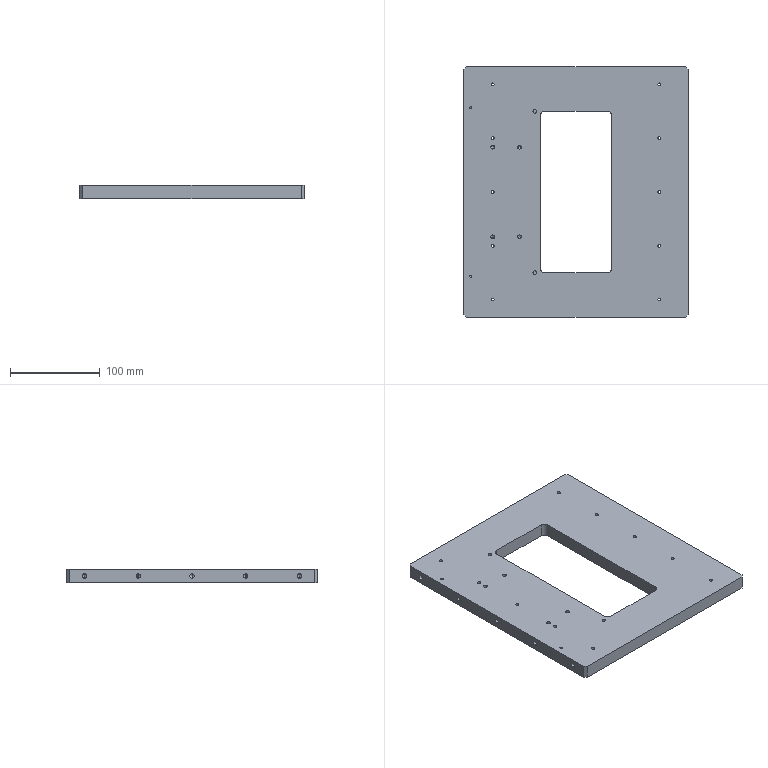Part | STEP file | 10-12 lift fixing plate A | 1 solid | 136 faces | box 250 x 280 x 15 mm | volume 827776 mm3 | cylinder 76 | cone 40 | plane 20 | commonest cylinder face diameters 3.3 x20 5 x20 4.2 x16 4 x12 2.5 x4 10 x4